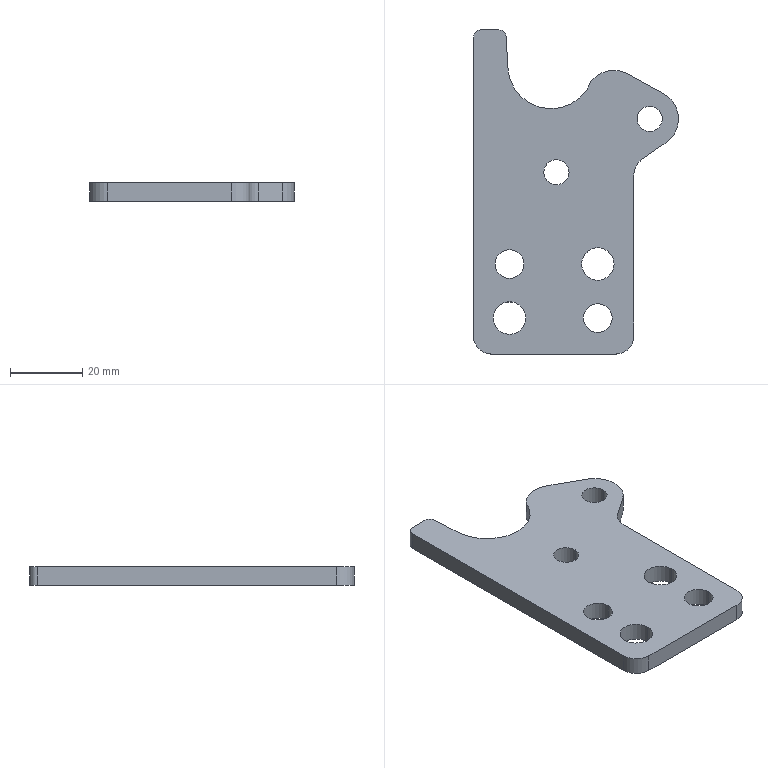Part | SolidWorks | features Fillet 2, Extrusion 1 | 1 solid | 29 faces | box 56.9 x 90 x 5 mm | volume 16455 mm3 | cylinder 20 | plane 9 | commonest cylinder face diameters 7 x4 8 x4 9 x4 4 x2 10 x2 16 x2
STEP:
#1=CARTESIAN_POINT('',(19.5,50.5,5.));
#2=VERTEX_POINT('',#1);
#3=CARTESIAN_POINT('',(26.5,50.5,5.));
#4=VERTEX_POINT('',#3);
#5=CARTESIAN_POINT('',(23.,50.5,5.));
#6=DIRECTION('',(0.,0.,1.));
#7=DIRECTION('',(1.,0.,0.));
#8=AXIS2_PLACEMENT_3D('',#5,#6,#7);
#9=CIRCLE('',#8,3.5);
#10=EDGE_CURVE('',#2,#4,#9,.T.);
#11=ORIENTED_EDGE('',*,*,#10,.T.);
#12=CARTESIAN_POINT('',(26.5,50.5,0.));
#13=VERTEX_POINT('',#12);
#14=CARTESIAN_POINT('',(26.5,50.5,5.));
#15=DIRECTION('',(0.,0.,-1.));
#16=VECTOR('',#15,1000.);
#17=LINE('',#14,#16);
#18=EDGE_CURVE('',#4,#13,#17,.T.);
#19=ORIENTED_EDGE('',*,*,#18,.T.);
#20=CARTESIAN_POINT('',(19.5,50.5,0.));
#21=VERTEX_POINT('',#20);
#22=CARTESIAN_POINT('',(23.,50.5,0.));
#23=DIRECTION('',(0.,0.,1.));
#24=DIRECTION('',(1.,0.,0.));
#25=AXIS2_PLACEMENT_3D('',#22,#23,#24);
#26=CIRCLE('',#25,3.5);
#27=EDGE_CURVE('',#21,#13,#26,.T.);
#28=ORIENTED_EDGE('',*,*,#27,.F.);
#29=CARTESIAN_POINT('',(19.5,50.5,5.));
#30=DIRECTION('',(0.,0.,-1.));
#31=VECTOR('',#30,1000.);
#32=LINE('',#29,#31);
#33=EDGE_CURVE('',#2,#21,#32,.T.);
#34=ORIENTED_EDGE('',*,*,#33,.F.);
#35=EDGE_LOOP('',(#11,#19,#28,#34));
#36=FACE_OUTER_BOUND('',#35,.T.);
#37=CARTESIAN_POINT('',(23.,50.5,5.));
#38=DIRECTION('',(0.,0.,-1.));
#39=DIRECTION('',(-1.,0.,0.));
#40=AXIS2_PLACEMENT_3D('',#37,#38,#39);
#41=CYLINDRICAL_SURFACE('',#40,3.5);
#42=ADVANCED_FACE('',(#36),#41,.F.);
#43=CARTESIAN_POINT('',(30.,25.,5.));
#44=VERTEX_POINT('',#43);
#45=CARTESIAN_POINT('',(39.,25.,5.));
#46=VERTEX_POINT('',#45);
#47=CARTESIAN_POINT('',(34.5,25.,5.));
#48=DIRECTION('',(0.,0.,1.));
#49=DIRECTION('',(1.,0.,0.));
#50=AXIS2_PLACEMENT_3D('',#47,#48,#49);
#51=CIRCLE('',#50,4.5);
#52=EDGE_CURVE('',#44,#46,#51,.T.);
#53=ORIENTED_EDGE('',*,*,#52,.T.);
#54=CARTESIAN_POINT('',(39.,25.,0.));
#55=VERTEX_POINT('',#54);
#56=CARTESIAN_POINT('',(39.,25.,5.));
#57=DIRECTION('',(0.,0.,-1.));
#58=VECTOR('',#57,1000.);
#59=LINE('',#56,#58);
#60=EDGE_CURVE('',#46,#55,#59,.T.);
#61=ORIENTED_EDGE('',*,*,#60,.T.);
#62=CARTESIAN_POINT('',(30.,25.,0.));
#63=VERTEX_POINT('',#62);
#64=CARTESIAN_POINT('',(34.5,25.,0.));
#65=DIRECTION('',(0.,0.,1.));
#66=DIRECTION('',(1.,0.,0.));
#67=AXIS2_PLACEMENT_3D('',#64,#65,#66);
#68=CIRCLE('',#67,4.5);
#69=EDGE_CURVE('',#63,#55,#68,.T.);
#70=ORIENTED_EDGE('',*,*,#69,.F.);
#71=CARTESIAN_POINT('',(30.,25.,5.));
#72=DIRECTION('',(0.,0.,-1.));
#73=VECTOR('',#72,1000.);
#74=LINE('',#71,#73);
#75=EDGE_CURVE('',#44,#63,#74,.T.);
#76=ORIENTED_EDGE('',*,*,#75,.F.);
#77=EDGE_LOOP('',(#53,#61,#70,#76));
#78=FACE_OUTER_BOUND('',#77,.T.);
#79=CARTESIAN_POINT('',(34.5,25.,5.));
#80=DIRECTION('',(0.,0.,-1.));
#81=DIRECTION('',(-1.,0.,0.));
#82=AXIS2_PLACEMENT_3D('',#79,#80,#81);
#83=CYLINDRICAL_SURFACE('',#82,4.5);
#84=ADVANCED_FACE('',(#78),#83,.F.);
#85=CARTESIAN_POINT('',(30.5,10.,5.));
#86=VERTEX_POINT('',#85);
#87=CARTESIAN_POINT('',(38.5,10.,5.));
#88=VERTEX_POINT('',#87);
#89=CARTESIAN_POINT('',(34.5,10.,5.));
#90=DIRECTION('',(0.,0.,1.));
#91=DIRECTION('',(1.,0.,0.));
#92=AXIS2_PLACEMENT_3D('',#89,#90,#91);
#93=CIRCLE('',#92,4.);
#94=EDGE_CURVE('',#86,#88,#93,.T.);
#95=ORIENTED_EDGE('',*,*,#94,.T.);
#96=CARTESIAN_POINT('',(38.5,10.,0.));
#97=VERTEX_POINT('',#96);
#98=CARTESIAN_POINT('',(38.5,10.,5.));
#99=DIRECTION('',(0.,0.,-1.));
#100=VECTOR('',#99,1000.);
#101=LINE('',#98,#100);
#102=EDGE_CURVE('',#88,#97,#101,.T.);
#103=ORIENTED_EDGE('',*,*,#102,.T.);
#104=CARTESIAN_POINT('',(30.5,10.,0.));
#105=VERTEX_POINT('',#104);
#106=CARTESIAN_POINT('',(34.5,10.,0.));
#107=DIRECTION('',(0.,0.,1.));
#108=DIRECTION('',(1.,0.,0.));
#109=AXIS2_PLACEMENT_3D('',#106,#107,#108);
#110=CIRCLE('',#109,4.);
#111=EDGE_CURVE('',#105,#97,#110,.T.);
#112=ORIENTED_EDGE('',*,*,#111,.F.);
#113=CARTESIAN_POINT('',(30.5,10.,5.));
#114=DIRECTION('',(0.,0.,-1.));
#115=VECTOR('',#114,1000.);
#116=LINE('',#113,#115);
#117=EDGE_CURVE('',#86,#105,#116,.T.);
#118=ORIENTED_EDGE('',*,*,#117,.F.);
#119=EDGE_LOOP('',(#95,#103,#112,#118));
#120=FACE_OUTER_BOUND('',#119,.T.);
#121=CARTESIAN_POINT('',(34.5,10.,5.));
#122=DIRECTION('',(0.,0.,-1.));
#123=DIRECTION('',(-1.,0.,0.));
#124=AXIS2_PLACEMENT_3D('',#121,#122,#123);
#125=CYLINDRICAL_SURFACE('',#124,4.);
#126=ADVANCED_FACE('',(#120),#125,.F.);
#127=CARTESIAN_POINT('',(6.,25.,5.));
#128=VERTEX_POINT('',#127);
#129=CARTESIAN_POINT('',(14.,25.,5.));
#130=VERTEX_POINT('',#129);
#131=CARTESIAN_POINT('',(10.,25.,5.));
#132=DIRECTION('',(0.,0.,1.));
#133=DIRECTION('',(1.,0.,0.));
#134=AXIS2_PLACEMENT_3D('',#131,#132,#133);
#135=CIRCLE('',#134,4.);
#136=EDGE_CURVE('',#128,#130,#135,.T.);
#137=ORIENTED_EDGE('',*,*,#136,.T.);
#138=CARTESIAN_POINT('',(14.,25.,0.));
#139=VERTEX_POINT('',#138);
#140=CARTESIAN_POINT('',(14.,25.,5.));
#141=DIRECTION('',(0.,0.,-1.));
#142=VECTOR('',#141,1000.);
#143=LINE('',#140,#142);
#144=EDGE_CURVE('',#130,#139,#143,.T.);
#145=ORIENTED_EDGE('',*,*,#144,.T.);
#146=CARTESIAN_POINT('',(6.,25.,0.));
#147=VERTEX_POINT('',#146);
#148=CARTESIAN_POINT('',(10.,25.,0.));
#149=DIRECTION('',(0.,0.,1.));
#150=DIRECTION('',(1.,0.,0.));
#151=AXIS2_PLACEMENT_3D('',#148,#149,#150);
#152=CIRCLE('',#151,4.);
#153=EDGE_CURVE('',#147,#139,#152,.T.);
#154=ORIENTED_EDGE('',*,*,#153,.F.);
#155=CARTESIAN_POINT('',(6.,25.,5.));
#156=DIRECTION('',(0.,0.,-1.));
#157=VECTOR('',#156,1000.);
#158=LINE('',#155,#157);
#159=EDGE_CURVE('',#128,#147,#158,.T.);
#160=ORIENTED_EDGE('',*,*,#159,.F.);
#161=EDGE_LOOP('',(#137,#145,#154,#160));
#162=FACE_OUTER_BOUND('',#161,.T.);
#163=CARTESIAN_POINT('',(10.,25.,5.));
#164=DIRECTION('',(0.,0.,-1.));
#165=DIRECTION('',(-1.,0.,0.));
#166=AXIS2_PLACEMENT_3D('',#163,#164,#165);
#167=CYLINDRICAL_SURFACE('',#166,4.);
#168=ADVANCED_FACE('',(#162),#167,.F.);
#169=CARTESIAN_POINT('',(5.5,10.,5.));
#170=VERTEX_POINT('',#169);
#171=CARTESIAN_POINT('',(14.5,10.,5.));
#172=VERTEX_POINT('',#171);
#173=CARTESIAN_POINT('',(10.,10.,5.));
#174=DIRECTION('',(0.,0.,1.));
#175=DIRECTION('',(1.,0.,0.));
#176=AXIS2_PLACEMENT_3D('',#173,#174,#175);
#177=CIRCLE('',#176,4.5);
#178=EDGE_CURVE('',#170,#172,#177,.T.);
#179=ORIENTED_EDGE('',*,*,#178,.T.);
#180=CARTESIAN_POINT('',(14.5,10.,0.));
#181=VERTEX_POINT('',#180);
#182=CARTESIAN_POINT('',(14.5,10.,5.));
#183=DIRECTION('',(0.,0.,-1.));
#184=VECTOR('',#183,1000.);
#185=LINE('',#182,#184);
#186=EDGE_CURVE('',#172,#181,#185,.T.);
#187=ORIENTED_EDGE('',*,*,#186,.T.);
#188=CARTESIAN_POINT('',(5.5,10.,0.));
#189=VERTEX_POINT('',#188);
#190=CARTESIAN_POINT('',(10.,10.,0.));
#191=DIRECTION('',(0.,0.,1.));
#192=DIRECTION('',(1.,0.,0.));
#193=AXIS2_PLACEMENT_3D('',#190,#191,#192);
#194=CIRCLE('',#193,4.5);
#195=EDGE_CURVE('',#189,#181,#194,.T.);
#196=ORIENTED_EDGE('',*,*,#195,.F.);
#197=CARTESIAN_POINT('',(5.5,10.,5.));
#198=DIRECTION('',(0.,0.,-1.));
#199=VECTOR('',#198,1000.);
#200=LINE('',#197,#199);
#201=EDGE_CURVE('',#170,#189,#200,.T.);
#202=ORIENTED_EDGE('',*,*,#201,.F.);
#203=EDGE_LOOP('',(#179,#187,#196,#202));
#204=FACE_OUTER_BOUND('',#203,.T.);
#205=CARTESIAN_POINT('',(10.,10.,5.));
#206=DIRECTION('',(0.,0.,-1.));
#207=DIRECTION('',(-1.,0.,0.));
#208=AXIS2_PLACEMENT_3D('',#205,#206,#207);
#209=CYLINDRICAL_SURFACE('',#208,4.5);
#210=ADVANCED_FACE('',(#204),#209,.F.);
#211=CARTESIAN_POINT('',(45.4,65.3,5.));
#212=VERTEX_POINT('',#211);
#213=CARTESIAN_POINT('',(52.4,65.3,5.));
#214=VERTEX_POINT('',#213);
#215=CARTESIAN_POINT('',(48.9,65.3,5.));
#216=DIRECTION('',(0.,0.,1.));
#217=DIRECTION('',(1.,0.,0.));
#218=AXIS2_PLACEMENT_3D('',#215,#216,#217);
#219=CIRCLE('',#218,3.5);
#220=EDGE_CURVE('',#212,#214,#219,.T.);
#221=ORIENTED_EDGE('',*,*,#220,.T.);
#222=CARTESIAN_POINT('',(52.4,65.3,0.));
#223=VERTEX_POINT('',#222);
#224=CARTESIAN_POINT('',(52.4,65.3,5.));
#225=DIRECTION('',(0.,0.,-1.));
#226=VECTOR('',#225,1000.);
#227=LINE('',#224,#226);
#228=EDGE_CURVE('',#214,#223,#227,.T.);
#229=ORIENTED_EDGE('',*,*,#228,.T.);
#230=CARTESIAN_POINT('',(45.4,65.3,0.));
#231=VERTEX_POINT('',#230);
#232=CARTESIAN_POINT('',(48.9,65.3,0.));
#233=DIRECTION('',(0.,0.,1.));
#234=DIRECTION('',(1.,0.,0.));
#235=AXIS2_PLACEMENT_3D('',#232,#233,#234);
#236=CIRCLE('',#235,3.5);
#237=EDGE_CURVE('',#231,#223,#236,.T.);
#238=ORIENTED_EDGE('',*,*,#237,.F.);
#239=CARTESIAN_POINT('',(45.4,65.3,5.));
#240=DIRECTION('',(0.,0.,-1.));
#241=VECTOR('',#240,1000.);
#242=LINE('',#239,#241);
#243=EDGE_CURVE('',#212,#231,#242,.T.);
#244=ORIENTED_EDGE('',*,*,#243,.F.);
#245=EDGE_LOOP('',(#221,#229,#238,#244));
#246=FACE_OUTER_BOUND('',#245,.T.);
#247=CARTESIAN_POINT('',(48.9,65.3,5.));
#248=DIRECTION('',(0.,0.,-1.));
#249=DIRECTION('',(-1.,0.,0.));
#250=AXIS2_PLACEMENT_3D('',#247,#248,#249);
#251=CYLINDRICAL_SURFACE('',#250,3.5);
#252=ADVANCED_FACE('',(#246),#251,.F.);
#253=ORIENTED_EDGE('',*,*,#52,.F.);
#254=CARTESIAN_POINT('',(34.5,25.,5.));
#255=DIRECTION('',(0.,0.,1.));
#256=DIRECTION('',(1.,0.,0.));
#257=AXIS2_PLACEMENT_3D('',#254,#255,#256);
#258=CIRCLE('',#257,4.5);
#259=EDGE_CURVE('',#46,#44,#258,.T.);
#260=ORIENTED_EDGE('',*,*,#259,.F.);
#261=EDGE_LOOP('',(#253,#260));
#262=FACE_BOUND('',#261,.T.);
#263=ORIENTED_EDGE('',*,*,#136,.F.);
#264=CARTESIAN_POINT('',(10.,25.,5.));
#265=DIRECTION('',(0.,0.,1.));
#266=DIRECTION('',(1.,0.,0.));
#267=AXIS2_PLACEMENT_3D('',#264,#265,#266);
#268=CIRCLE('',#267,4.);
#269=EDGE_CURVE('',#130,#128,#268,.T.);
#270=ORIENTED_EDGE('',*,*,#269,.F.);
#271=EDGE_LOOP('',(#263,#270));
#272=FACE_BOUND('',#271,.T.);
#273=ORIENTED_EDGE('',*,*,#220,.F.);
#274=CARTESIAN_POINT('',(48.9,65.3,5.));
#275=DIRECTION('',(0.,0.,1.));
#276=DIRECTION('',(1.,0.,0.));
#277=AXIS2_PLACEMENT_3D('',#274,#275,#276);
#278=CIRCLE('',#277,3.5);
#279=EDGE_CURVE('',#214,#212,#278,.T.);
#280=ORIENTED_EDGE('',*,*,#279,.F.);
#281=EDGE_LOOP('',(#273,#280));
#282=FACE_BOUND('',#281,.T.);
#283=CARTESIAN_POINT('',(5.,0.,5.));
#284=VERTEX_POINT('',#283);
#285=CARTESIAN_POINT('',(39.5,0.,5.));
#286=VERTEX_POINT('',#285);
#287=CARTESIAN_POINT('',(0.,0.,5.));
#288=DIRECTION('',(1.,0.,0.));
#289=VECTOR('',#288,1000.);
#290=LINE('',#287,#289);
#291=EDGE_CURVE('',#284,#286,#290,.T.);
#292=ORIENTED_EDGE('',*,*,#291,.T.);
#293=CARTESIAN_POINT('',(44.5,5.,5.));
#294=VERTEX_POINT('',#293);
#295=CARTESIAN_POINT('',(39.5,5.,5.));
#296=DIRECTION('',(0.,0.,1.));
#297=DIRECTION('',(1.,0.,0.));
#298=AXIS2_PLACEMENT_3D('',#295,#296,#297);
#299=CIRCLE('',#298,5.);
#300=EDGE_CURVE('',#286,#294,#299,.T.);
#301=ORIENTED_EDGE('',*,*,#300,.T.);
#302=CARTESIAN_POINT('',(44.5,49.666,5.));
#303=VERTEX_POINT('',#302);
#304=CARTESIAN_POINT('',(44.5,0.,5.));
#305=DIRECTION('',(0.,1.,0.));
#306=VECTOR('',#305,1000.);
#307=LINE('',#304,#306);
#308=EDGE_CURVE('',#294,#303,#307,.T.);
#309=ORIENTED_EDGE('',*,*,#308,.T.);
#310=CARTESIAN_POINT('',(46.881,54.196,5.));
#311=VERTEX_POINT('',#310);
#312=CARTESIAN_POINT('',(50.,49.666,5.));
#313=DIRECTION('',(0.,0.,-1.));
#314=DIRECTION('',(1.,0.,0.));
#315=AXIS2_PLACEMENT_3D('',#312,#313,#314);
#316=CIRCLE('',#315,5.5);
#317=EDGE_CURVE('',#303,#311,#316,.T.);
#318=ORIENTED_EDGE('',*,*,#317,.T.);
#319=CARTESIAN_POINT('',(53.437,58.711,5.));
#320=VERTEX_POINT('',#319);
#321=CARTESIAN_POINT('',(53.437,58.711,5.));
#322=DIRECTION('',(0.8236,0.5672,0.));
#323=VECTOR('',#322,1000.);
#324=LINE('',#321,#323);
#325=EDGE_CURVE('',#311,#320,#324,.T.);
#326=ORIENTED_EDGE('',*,*,#325,.T.);
#327=CARTESIAN_POINT('',(52.755,72.31,5.));
#328=VERTEX_POINT('',#327);
#329=CARTESIAN_POINT('',(48.9,65.3,5.));
#330=DIRECTION('',(0.,0.,1.));
#331=DIRECTION('',(1.,0.,0.));
#332=AXIS2_PLACEMENT_3D('',#329,#330,#331);
#333=CIRCLE('',#332,8.);
#334=EDGE_CURVE('',#320,#328,#333,.T.);
#335=ORIENTED_EDGE('',*,*,#334,.T.);
#336=CARTESIAN_POINT('',(42.755,77.81,5.));
#337=VERTEX_POINT('',#336);
#338=CARTESIAN_POINT('',(42.755,77.81,5.));
#339=DIRECTION('',(-0.8762,0.4819,0.));
#340=VECTOR('',#339,1000.);
#341=LINE('',#338,#340);
#342=EDGE_CURVE('',#328,#337,#341,.T.);
#343=ORIENTED_EDGE('',*,*,#342,.T.);
#344=CARTESIAN_POINT('',(32.745,75.91,5.));
#345=VERTEX_POINT('',#344);
#346=CARTESIAN_POINT('',(38.9,70.8,5.));
#347=DIRECTION('',(0.,0.,1.));
#348=DIRECTION('',(1.,0.,0.));
#349=AXIS2_PLACEMENT_3D('',#346,#347,#348);
#350=CIRCLE('',#349,8.);
#351=EDGE_CURVE('',#337,#345,#350,.T.);
#352=ORIENTED_EDGE('',*,*,#351,.T.);
#353=CARTESIAN_POINT('',(9.516,79.472,5.));
#354=VERTEX_POINT('',#353);
#355=CARTESIAN_POINT('',(21.5,80.1,5.));
#356=DIRECTION('',(0.,0.,-1.));
#357=DIRECTION('',(1.,0.,0.));
#358=AXIS2_PLACEMENT_3D('',#355,#356,#357);
#359=CIRCLE('',#358,12.);
#360=EDGE_CURVE('',#345,#354,#359,.T.);
#361=ORIENTED_EDGE('',*,*,#360,.T.);
#362=CARTESIAN_POINT('',(9.064,88.105,5.));
#363=VERTEX_POINT('',#362);
#364=CARTESIAN_POINT('',(8.965,90.,5.));
#365=DIRECTION('',(-0.05234,0.9986,0.));
#366=VECTOR('',#365,1000.);
#367=LINE('',#364,#366);
#368=EDGE_CURVE('',#354,#363,#367,.T.);
#369=ORIENTED_EDGE('',*,*,#368,.T.);
#370=CARTESIAN_POINT('',(7.067,90.,5.));
#371=VERTEX_POINT('',#370);
#372=CARTESIAN_POINT('',(7.067,88.,5.));
#373=DIRECTION('',(0.,0.,1.));
#374=DIRECTION('',(1.,0.,0.));
#375=AXIS2_PLACEMENT_3D('',#372,#373,#374);
#376=CIRCLE('',#375,2.);
#377=EDGE_CURVE('',#363,#371,#376,.T.);
#378=ORIENTED_EDGE('',*,*,#377,.T.);
#379=CARTESIAN_POINT('',(2.,90.,5.));
#380=VERTEX_POINT('',#379);
#381=CARTESIAN_POINT('',(0.,90.,5.));
#382=DIRECTION('',(-1.,0.,0.));
#383=VECTOR('',#382,1000.);
#384=LINE('',#381,#383);
#385=EDGE_CURVE('',#371,#380,#384,.T.);
#386=ORIENTED_EDGE('',*,*,#385,.T.);
#387=CARTESIAN_POINT('',(0.,88.,5.));
#388=VERTEX_POINT('',#387);
#389=CARTESIAN_POINT('',(2.,88.,5.));
#390=DIRECTION('',(0.,0.,1.));
#391=DIRECTION('',(1.,0.,0.));
#392=AXIS2_PLACEMENT_3D('',#389,#390,#391);
#393=CIRCLE('',#392,2.);
#394=EDGE_CURVE('',#380,#388,#393,.T.);
#395=ORIENTED_EDGE('',*,*,#394,.T.);
#396=CARTESIAN_POINT('',(0.,5.,5.));
#397=VERTEX_POINT('',#396);
#398=CARTESIAN_POINT('',(0.,0.,5.));
#399=DIRECTION('',(0.,-1.,0.));
#400=VECTOR('',#399,1000.);
#401=LINE('',#398,#400);
#402=EDGE_CURVE('',#388,#397,#401,.T.);
#403=ORIENTED_EDGE('',*,*,#402,.T.);
#404=CARTESIAN_POINT('',(5.,5.,5.));
#405=DIRECTION('',(0.,0.,1.));
#406=DIRECTION('',(1.,0.,0.));
#407=AXIS2_PLACEMENT_3D('',#404,#405,#406);
#408=CIRCLE('',#407,5.);
#409=EDGE_CURVE('',#397,#284,#408,.T.);
#410=ORIENTED_EDGE('',*,*,#409,.T.);
#411=EDGE_LOOP('',(#292,#301,#309,#318,#326,#335,#343,#352,#361,#369,#378,#386,#395,#403,#410));
#412=FACE_OUTER_BOUND('',#411,.T.);
#413=ORIENTED_EDGE('',*,*,#178,.F.);
#414=CARTESIAN_POINT('',(10.,10.,5.));
#415=DIRECTION('',(0.,0.,1.));
#416=DIRECTION('',(1.,0.,0.));
#417=AXIS2_PLACEMENT_3D('',#414,#415,#416);
#418=CIRCLE('',#417,4.5);
#419=EDGE_CURVE('',#172,#170,#418,.T.);
#420=ORIENTED_EDGE('',*,*,#419,.F.);
#421=EDGE_LOOP('',(#413,#420));
#422=FACE_BOUND('',#421,.T.);
#423=ORIENTED_EDGE('',*,*,#94,.F.);
#424=CARTESIAN_POINT('',(34.5,10.,5.));
#425=DIRECTION('',(0.,0.,1.));
#426=DIRECTION('',(1.,0.,0.));
#427=AXIS2_PLACEMENT_3D('',#424,#425,#426);
#428=CIRCLE('',#427,4.);
#429=EDGE_CURVE('',#88,#86,#428,.T.);
#430=ORIENTED_EDGE('',*,*,#429,.F.);
#431=EDGE_LOOP('',(#423,#430));
#432=FACE_BOUND('',#431,.T.);
#433=ORIENTED_EDGE('',*,*,#10,.F.);
#434=CARTESIAN_POINT('',(23.,50.5,5.));
#435=DIRECTION('',(0.,0.,1.));
#436=DIRECTION('',(1.,0.,0.));
#437=AXIS2_PLACEMENT_3D('',#434,#435,#436);
#438=CIRCLE('',#437,3.5);
#439=EDGE_CURVE('',#4,#2,#438,.T.);
#440=ORIENTED_EDGE('',*,*,#439,.F.);
#441=EDGE_LOOP('',(#433,#440));
#442=FACE_BOUND('',#441,.T.);
#443=CARTESIAN_POINT('',(21.5,80.1,5.));
#444=DIRECTION('',(0.,0.,1.));
#445=DIRECTION('',(1.,0.,0.));
#446=AXIS2_PLACEMENT_3D('',#443,#444,#445);
#447=PLANE('',#446);
#448=ADVANCED_FACE('',(#262,#272,#282,#412,#422,#432,#442),#447,.T.);
#449=CARTESIAN_POINT('',(44.5,5.,0.));
#450=VERTEX_POINT('',#449);
#451=CARTESIAN_POINT('',(44.5,49.666,0.));
#452=VERTEX_POINT('',#451);
#453=CARTESIAN_POINT('',(44.5,0.,0.));
#454=DIRECTION('',(0.,1.,0.));
#455=VECTOR('',#454,1000.);
#456=LINE('',#453,#455);
#457=EDGE_CURVE('',#450,#452,#456,.T.);
#458=ORIENTED_EDGE('',*,*,#457,.F.);
#459=CARTESIAN_POINT('',(39.5,0.,0.));
#460=VERTEX_POINT('',#459);
#461=CARTESIAN_POINT('',(39.5,5.,0.));
#462=DIRECTION('',(0.,0.,-1.));
#463=DIRECTION('',(1.,0.,0.));
#464=AXIS2_PLACEMENT_3D('',#461,#462,#463);
#465=CIRCLE('',#464,5.);
#466=EDGE_CURVE('',#450,#460,#465,.T.);
#467=ORIENTED_EDGE('',*,*,#466,.T.);
#468=CARTESIAN_POINT('',(5.,0.,0.));
#469=VERTEX_POINT('',#468);
#470=CARTESIAN_POINT('',(0.,0.,0.));
#471=DIRECTION('',(1.,0.,0.));
#472=VECTOR('',#471,1000.);
#473=LINE('',#470,#472);
#474=EDGE_CURVE('',#469,#460,#473,.T.);
#475=ORIENTED_EDGE('',*,*,#474,.F.);
#476=CARTESIAN_POINT('',(0.,5.,0.));
#477=VERTEX_POINT('',#476);
#478=CARTESIAN_POINT('',(5.,5.,0.));
#479=DIRECTION('',(0.,0.,-1.));
#480=DIRECTION('',(1.,0.,0.));
#481=AXIS2_PLACEMENT_3D('',#478,#479,#480);
#482=CIRCLE('',#481,5.);
#483=EDGE_CURVE('',#469,#477,#482,.T.);
#484=ORIENTED_EDGE('',*,*,#483,.T.);
#485=CARTESIAN_POINT('',(0.,88.,0.));
#486=VERTEX_POINT('',#485);
#487=CARTESIAN_POINT('',(0.,0.,0.));
#488=DIRECTION('',(0.,-1.,0.));
#489=VECTOR('',#488,1000.);
#490=LINE('',#487,#489);
#491=EDGE_CURVE('',#486,#477,#490,.T.);
#492=ORIENTED_EDGE('',*,*,#491,.F.);
#493=CARTESIAN_POINT('',(2.,90.,0.));
#494=VERTEX_POINT('',#493);
#495=CARTESIAN_POINT('',(2.,88.,0.));
#496=DIRECTION('',(0.,0.,-1.));
#497=DIRECTION('',(1.,0.,0.));
#498=AXIS2_PLACEMENT_3D('',#495,#496,#497);
#499=CIRCLE('',#498,2.);
#500=EDGE_CURVE('',#486,#494,#499,.T.);
#501=ORIENTED_EDGE('',*,*,#500,.T.);
#502=CARTESIAN_POINT('',(7.067,90.,0.));
#503=VERTEX_POINT('',#502);
#504=CARTESIAN_POINT('',(0.,90.,0.));
#505=DIRECTION('',(-1.,0.,0.));
#506=VECTOR('',#505,1000.);
#507=LINE('',#504,#506);
#508=EDGE_CURVE('',#503,#494,#507,.T.);
#509=ORIENTED_EDGE('',*,*,#508,.F.);
#510=CARTESIAN_POINT('',(9.064,88.105,0.));
#511=VERTEX_POINT('',#510);
#512=CARTESIAN_POINT('',(7.067,88.,0.));
#513=DIRECTION('',(0.,0.,-1.));
#514=DIRECTION('',(1.,0.,0.));
#515=AXIS2_PLACEMENT_3D('',#512,#513,#514);
#516=CIRCLE('',#515,2.);
#517=EDGE_CURVE('',#503,#511,#516,.T.);
#518=ORIENTED_EDGE('',*,*,#517,.T.);
#519=CARTESIAN_POINT('',(9.516,79.472,0.));
#520=VERTEX_POINT('',#519);
#521=CARTESIAN_POINT('',(8.965,90.,0.));
#522=DIRECTION('',(-0.05234,0.9986,0.));
#523=VECTOR('',#522,1000.);
#524=LINE('',#521,#523);
#525=EDGE_CURVE('',#520,#511,#524,.T.);
#526=ORIENTED_EDGE('',*,*,#525,.F.);
#527=CARTESIAN_POINT('',(32.745,75.91,0.));
#528=VERTEX_POINT('',#527);
#529=CARTESIAN_POINT('',(21.5,80.1,0.));
#530=DIRECTION('',(0.,0.,-1.));
#531=DIRECTION('',(1.,0.,0.));
#532=AXIS2_PLACEMENT_3D('',#529,#530,#531);
#533=CIRCLE('',#532,12.);
#534=EDGE_CURVE('',#528,#520,#533,.T.);
#535=ORIENTED_EDGE('',*,*,#534,.F.);
#536=CARTESIAN_POINT('',(42.755,77.81,0.));
#537=VERTEX_POINT('',#536);
#538=CARTESIAN_POINT('',(38.9,70.8,0.));
#539=DIRECTION('',(0.,0.,1.));
#540=DIRECTION('',(1.,0.,0.));
#541=AXIS2_PLACEMENT_3D('',#538,#539,#540);
#542=CIRCLE('',#541,8.);
#543=EDGE_CURVE('',#537,#528,#542,.T.);
#544=ORIENTED_EDGE('',*,*,#543,.F.);
#545=CARTESIAN_POINT('',(52.755,72.31,0.));
#546=VERTEX_POINT('',#545);
#547=CARTESIAN_POINT('',(42.755,77.81,0.));
#548=DIRECTION('',(-0.8762,0.4819,0.));
#549=VECTOR('',#548,1000.);
#550=LINE('',#547,#549);
#551=EDGE_CURVE('',#546,#537,#550,.T.);
#552=ORIENTED_EDGE('',*,*,#551,.F.);
#553=CARTESIAN_POINT('',(53.437,58.711,0.));
#554=VERTEX_POINT('',#553);
#555=CARTESIAN_POINT('',(48.9,65.3,0.));
#556=DIRECTION('',(0.,0.,1.));
#557=DIRECTION('',(1.,0.,0.));
#558=AXIS2_PLACEMENT_3D('',#555,#556,#557);
#559=CIRCLE('',#558,8.);
#560=EDGE_CURVE('',#554,#546,#559,.T.);
#561=ORIENTED_EDGE('',*,*,#560,.F.);
#562=CARTESIAN_POINT('',(46.881,54.196,0.));
#563=VERTEX_POINT('',#562);
#564=CARTESIAN_POINT('',(53.437,58.711,0.));
#565=DIRECTION('',(0.8236,0.5672,0.));
#566=VECTOR('',#565,1000.);
#567=LINE('',#564,#566);
#568=EDGE_CURVE('',#563,#554,#567,.T.);
#569=ORIENTED_EDGE('',*,*,#568,.F.);
#570=CARTESIAN_POINT('',(50.,49.666,0.));
#571=DIRECTION('',(0.,0.,-1.));
#572=DIRECTION('',(1.,0.,0.));
#573=AXIS2_PLACEMENT_3D('',#570,#571,#572);
#574=CIRCLE('',#573,5.5);
#575=EDGE_CURVE('',#452,#563,#574,.T.);
#576=ORIENTED_EDGE('',*,*,#575,.F.);
#577=EDGE_LOOP('',(#458,#467,#475,#484,#492,#501,#509,#518,#526,#535,#544,#552,#561,#569,#576));
#578=FACE_OUTER_BOUND('',#577,.T.);
#579=ORIENTED_EDGE('',*,*,#237,.T.);
#580=CARTESIAN_POINT('',(48.9,65.3,0.));
#581=DIRECTION('',(0.,0.,1.));
#582=DIRECTION('',(1.,0.,0.));
#583=AXIS2_PLACEMENT_3D('',#580,#581,#582);
#584=CIRCLE('',#583,3.5);
#585=EDGE_CURVE('',#223,#231,#584,.T.);
#586=ORIENTED_EDGE('',*,*,#585,.T.);
#587=EDGE_LOOP('',(#579,#586));
#588=FACE_BOUND('',#587,.T.);
#589=ORIENTED_EDGE('',*,*,#195,.T.);
#590=CARTESIAN_POINT('',(10.,10.,0.));
#591=DIRECTION('',(0.,0.,1.));
#592=DIRECTION('',(1.,0.,0.));
#593=AXIS2_PLACEMENT_3D('',#590,#591,#592);
#594=CIRCLE('',#593,4.5);
#595=EDGE_CURVE('',#181,#189,#594,.T.);
#596=ORIENTED_EDGE('',*,*,#595,.T.);
#597=EDGE_LOOP('',(#589,#596));
#598=FACE_BOUND('',#597,.T.);
#599=ORIENTED_EDGE('',*,*,#153,.T.);
#600=CARTESIAN_POINT('',(10.,25.,0.));
#601=DIRECTION('',(0.,0.,1.));
#602=DIRECTION('',(1.,0.,0.));
#603=AXIS2_PLACEMENT_3D('',#600,#601,#602);
#604=CIRCLE('',#603,4.);
#605=EDGE_CURVE('',#139,#147,#604,.T.);
#606=ORIENTED_EDGE('',*,*,#605,.T.);
#607=EDGE_LOOP('',(#599,#606));
#608=FACE_BOUND('',#607,.T.);
#609=ORIENTED_EDGE('',*,*,#111,.T.);
#610=CARTESIAN_POINT('',(34.5,10.,0.));
#611=DIRECTION('',(0.,0.,1.));
#612=DIRECTION('',(1.,0.,0.));
#613=AXIS2_PLACEMENT_3D('',#610,#611,#612);
#614=CIRCLE('',#613,4.);
#615=EDGE_CURVE('',#97,#105,#614,.T.);
#616=ORIENTED_EDGE('',*,*,#615,.T.);
#617=EDGE_LOOP('',(#609,#616));
#618=FACE_BOUND('',#617,.T.);
#619=ORIENTED_EDGE('',*,*,#69,.T.);
#620=CARTESIAN_POINT('',(34.5,25.,0.));
#621=DIRECTION('',(0.,0.,1.));
#622=DIRECTION('',(1.,0.,0.));
#623=AXIS2_PLACEMENT_3D('',#620,#621,#622);
#624=CIRCLE('',#623,4.5);
#625=EDGE_CURVE('',#55,#63,#624,.T.);
#626=ORIENTED_EDGE('',*,*,#625,.T.);
#627=EDGE_LOOP('',(#619,#626));
#628=FACE_BOUND('',#627,.T.);
#629=ORIENTED_EDGE('',*,*,#27,.T.);
#630=CARTESIAN_POINT('',(23.,50.5,0.));
#631=DIRECTION('',(0.,0.,1.));
#632=DIRECTION('',(1.,0.,0.));
#633=AXIS2_PLACEMENT_3D('',#630,#631,#632);
#634=CIRCLE('',#633,3.5);
#635=EDGE_CURVE('',#13,#21,#634,.T.);
#636=ORIENTED_EDGE('',*,*,#635,.T.);
#637=EDGE_LOOP('',(#629,#636));
#638=FACE_BOUND('',#637,.T.);
#639=CARTESIAN_POINT('',(21.5,80.1,0.));
#640=DIRECTION('',(0.,0.,1.));
#641=DIRECTION('',(1.,0.,0.));
#642=AXIS2_PLACEMENT_3D('',#639,#640,#641);
#643=PLANE('',#642);
#644=ADVANCED_FACE('',(#578,#588,#598,#608,#618,#628,#638),#643,.F.);
#645=ORIENTED_EDGE('',*,*,#491,.T.);
#646=CARTESIAN_POINT('',(0.,5.,5.));
#647=DIRECTION('',(0.,0.,1.));
#648=VECTOR('',#647,1000.);
#649=LINE('',#646,#648);
#650=EDGE_CURVE('',#477,#397,#649,.T.);
#651=ORIENTED_EDGE('',*,*,#650,.T.);
#652=ORIENTED_EDGE('',*,*,#402,.F.);
#653=CARTESIAN_POINT('',(0.,88.,5.));
#654=DIRECTION('',(0.,0.,-1.));
#655=VECTOR('',#654,1000.);
#656=LINE('',#653,#655);
#657=EDGE_CURVE('',#388,#486,#656,.T.);
#658=ORIENTED_EDGE('',*,*,#657,.T.);
#659=EDGE_LOOP('',(#645,#651,#652,#658));
#660=FACE_OUTER_BOUND('',#659,.T.);
#661=CARTESIAN_POINT('',(0.,0.,5.));
#662=DIRECTION('',(1.,0.,0.));
#663=DIRECTION('',(0.,0.,-1.));
#664=AXIS2_PLACEMENT_3D('',#661,#662,#663);
#665=PLANE('',#664);
#666=ADVANCED_FACE('',(#660),#665,.F.);
#667=ORIENTED_EDGE('',*,*,#474,.T.);
#668=CARTESIAN_POINT('',(39.5,0.,5.));
#669=DIRECTION('',(0.,0.,1.));
#670=VECTOR('',#669,1000.);
#671=LINE('',#668,#670);
#672=EDGE_CURVE('',#460,#286,#671,.T.);
#673=ORIENTED_EDGE('',*,*,#672,.T.);
#674=ORIENTED_EDGE('',*,*,#291,.F.);
#675=CARTESIAN_POINT('',(5.,0.,5.));
#676=DIRECTION('',(0.,0.,-1.));
#677=VECTOR('',#676,1000.);
#678=LINE('',#675,#677);
#679=EDGE_CURVE('',#284,#469,#678,.T.);
#680=ORIENTED_EDGE('',*,*,#679,.T.);
#681=EDGE_LOOP('',(#667,#673,#674,#680));
#682=FACE_OUTER_BOUND('',#681,.T.);
#683=CARTESIAN_POINT('',(0.,0.,5.));
#684=DIRECTION('',(0.,1.,0.));
#685=DIRECTION('',(0.,0.,1.));
#686=AXIS2_PLACEMENT_3D('',#683,#684,#685);
#687=PLANE('',#686);
#688=ADVANCED_FACE('',(#682),#687,.F.);
#689=ORIENTED_EDGE('',*,*,#308,.F.);
#690=CARTESIAN_POINT('',(44.5,5.,5.));
#691=DIRECTION('',(0.,0.,-1.));
#692=VECTOR('',#691,1000.);
#693=LINE('',#690,#692);
#694=EDGE_CURVE('',#294,#450,#693,.T.);
#695=ORIENTED_EDGE('',*,*,#694,.T.);
#696=ORIENTED_EDGE('',*,*,#457,.T.);
#697=CARTESIAN_POINT('',(44.5,49.666,5.));
#698=DIRECTION('',(0.,0.,-1.));
#699=VECTOR('',#698,1000.);
#700=LINE('',#697,#699);
#701=EDGE_CURVE('',#303,#452,#700,.T.);
#702=ORIENTED_EDGE('',*,*,#701,.F.);
#703=EDGE_LOOP('',(#689,#695,#696,#702));
#704=FACE_OUTER_BOUND('',#703,.T.);
#705=CARTESIAN_POINT('',(44.5,0.,5.));
#706=DIRECTION('',(-1.,0.,0.));
#707=DIRECTION('',(0.,0.,1.));
#708=AXIS2_PLACEMENT_3D('',#705,#706,#707);
#709=PLANE('',#708);
#710=ADVANCED_FACE('',(#704),#709,.F.);
#711=ORIENTED_EDGE('',*,*,#575,.T.);
#712=CARTESIAN_POINT('',(46.881,54.196,5.));
#713=DIRECTION('',(0.,0.,-1.));
#714=VECTOR('',#713,1000.);
#715=LINE('',#712,#714);
#716=EDGE_CURVE('',#311,#563,#715,.T.);
#717=ORIENTED_EDGE('',*,*,#716,.F.);
#718=ORIENTED_EDGE('',*,*,#317,.F.);
#719=ORIENTED_EDGE('',*,*,#701,.T.);
#720=EDGE_LOOP('',(#711,#717,#718,#719));
#721=FACE_OUTER_BOUND('',#720,.T.);
#722=CARTESIAN_POINT('',(50.,49.666,5.));
#723=DIRECTION('',(0.,0.,-1.));
#724=DIRECTION('',(-1.,0.,0.));
#725=AXIS2_PLACEMENT_3D('',#722,#723,#724);
#726=CYLINDRICAL_SURFACE('',#725,5.5);
#727=ADVANCED_FACE('',(#721),#726,.F.);
#728=ORIENTED_EDGE('',*,*,#568,.T.);
#729=CARTESIAN_POINT('',(53.437,58.711,5.));
#730=DIRECTION('',(0.,0.,-1.));
#731=VECTOR('',#730,1000.);
#732=LINE('',#729,#731);
#733=EDGE_CURVE('',#320,#554,#732,.T.);
#734=ORIENTED_EDGE('',*,*,#733,.F.);
#735=ORIENTED_EDGE('',*,*,#325,.F.);
#736=ORIENTED_EDGE('',*,*,#716,.T.);
#737=EDGE_LOOP('',(#728,#734,#735,#736));
#738=FACE_OUTER_BOUND('',#737,.T.);
#739=CARTESIAN_POINT('',(53.437,58.711,5.));
#740=DIRECTION('',(-0.5672,0.8236,0.));
#741=DIRECTION('',(-0.8236,-0.5672,0.));
#742=AXIS2_PLACEMENT_3D('',#739,#740,#741);
#743=PLANE('',#742);
#744=ADVANCED_FACE('',(#738),#743,.F.);
#745=ORIENTED_EDGE('',*,*,#560,.T.);
#746=CARTESIAN_POINT('',(52.755,72.31,5.));
#747=DIRECTION('',(0.,0.,-1.));
#748=VECTOR('',#747,1000.);
#749=LINE('',#746,#748);
#750=EDGE_CURVE('',#328,#546,#749,.T.);
#751=ORIENTED_EDGE('',*,*,#750,.F.);
#752=ORIENTED_EDGE('',*,*,#334,.F.);
#753=ORIENTED_EDGE('',*,*,#733,.T.);
#754=EDGE_LOOP('',(#745,#751,#752,#753));
#755=FACE_OUTER_BOUND('',#754,.T.);
#756=CARTESIAN_POINT('',(48.9,65.3,5.));
#757=DIRECTION('',(0.,0.,-1.));
#758=DIRECTION('',(-1.,0.,0.));
#759=AXIS2_PLACEMENT_3D('',#756,#757,#758);
#760=CYLINDRICAL_SURFACE('',#759,8.);
#761=ADVANCED_FACE('',(#755),#760,.T.);
#762=ORIENTED_EDGE('',*,*,#551,.T.);
#763=CARTESIAN_POINT('',(42.755,77.81,5.));
#764=DIRECTION('',(0.,0.,-1.));
#765=VECTOR('',#764,1000.);
#766=LINE('',#763,#765);
#767=EDGE_CURVE('',#337,#537,#766,.T.);
#768=ORIENTED_EDGE('',*,*,#767,.F.);
#769=ORIENTED_EDGE('',*,*,#342,.F.);
#770=ORIENTED_EDGE('',*,*,#750,.T.);
#771=EDGE_LOOP('',(#762,#768,#769,#770));
#772=FACE_OUTER_BOUND('',#771,.T.);
#773=CARTESIAN_POINT('',(42.755,77.81,5.));
#774=DIRECTION('',(-0.4819,-0.8762,0.));
#775=DIRECTION('',(0.8762,-0.4819,0.));
#776=AXIS2_PLACEMENT_3D('',#773,#774,#775);
#777=PLANE('',#776);
#778=ADVANCED_FACE('',(#772),#777,.F.);
#779=ORIENTED_EDGE('',*,*,#543,.T.);
#780=CARTESIAN_POINT('',(32.745,75.91,5.));
#781=DIRECTION('',(0.,0.,-1.));
#782=VECTOR('',#781,1000.);
#783=LINE('',#780,#782);
#784=EDGE_CURVE('',#345,#528,#783,.T.);
#785=ORIENTED_EDGE('',*,*,#784,.F.);
#786=ORIENTED_EDGE('',*,*,#351,.F.);
#787=ORIENTED_EDGE('',*,*,#767,.T.);
#788=EDGE_LOOP('',(#779,#785,#786,#787));
#789=FACE_OUTER_BOUND('',#788,.T.);
#790=CARTESIAN_POINT('',(38.9,70.8,5.));
#791=DIRECTION('',(0.,0.,-1.));
#792=DIRECTION('',(-1.,0.,0.));
#793=AXIS2_PLACEMENT_3D('',#790,#791,#792);
#794=CYLINDRICAL_SURFACE('',#793,8.);
#795=ADVANCED_FACE('',(#789),#794,.T.);
#796=ORIENTED_EDGE('',*,*,#534,.T.);
#797=CARTESIAN_POINT('',(9.516,79.472,5.));
#798=DIRECTION('',(0.,0.,-1.));
#799=VECTOR('',#798,1000.);
#800=LINE('',#797,#799);
#801=EDGE_CURVE('',#354,#520,#800,.T.);
#802=ORIENTED_EDGE('',*,*,#801,.F.);
#803=ORIENTED_EDGE('',*,*,#360,.F.);
#804=ORIENTED_EDGE('',*,*,#784,.T.);
#805=EDGE_LOOP('',(#796,#802,#803,#804));
#806=FACE_OUTER_BOUND('',#805,.T.);
#807=CARTESIAN_POINT('',(21.5,80.1,5.));
#808=DIRECTION('',(0.,0.,-1.));
#809=DIRECTION('',(-1.,0.,0.));
#810=AXIS2_PLACEMENT_3D('',#807,#808,#809);
#811=CYLINDRICAL_SURFACE('',#810,12.);
#812=ADVANCED_FACE('',(#806),#811,.F.);
#813=ORIENTED_EDGE('',*,*,#525,.T.);
#814=CARTESIAN_POINT('',(9.064,88.105,5.));
#815=DIRECTION('',(0.,0.,1.));
#816=VECTOR('',#815,1000.);
#817=LINE('',#814,#816);
#818=EDGE_CURVE('',#511,#363,#817,.T.);
#819=ORIENTED_EDGE('',*,*,#818,.T.);
#820=ORIENTED_EDGE('',*,*,#368,.F.);
#821=ORIENTED_EDGE('',*,*,#801,.T.);
#822=EDGE_LOOP('',(#813,#819,#820,#821));
#823=FACE_OUTER_BOUND('',#822,.T.);
#824=CARTESIAN_POINT('',(8.965,90.,5.));
#825=DIRECTION('',(-0.9986,-0.05234,0.));
#826=DIRECTION('',(0.05234,-0.9986,0.));
#827=AXIS2_PLACEMENT_3D('',#824,#825,#826);
#828=PLANE('',#827);
#829=ADVANCED_FACE('',(#823),#828,.F.);
#830=ORIENTED_EDGE('',*,*,#385,.F.);
#831=CARTESIAN_POINT('',(7.067,90.,5.));
#832=DIRECTION('',(0.,0.,-1.));
#833=VECTOR('',#832,1000.);
#834=LINE('',#831,#833);
#835=EDGE_CURVE('',#371,#503,#834,.T.);
#836=ORIENTED_EDGE('',*,*,#835,.T.);
#837=ORIENTED_EDGE('',*,*,#508,.T.);
#838=CARTESIAN_POINT('',(2.,90.,5.));
#839=DIRECTION('',(0.,0.,1.));
#840=VECTOR('',#839,1000.);
#841=LINE('',#838,#840);
#842=EDGE_CURVE('',#494,#380,#841,.T.);
#843=ORIENTED_EDGE('',*,*,#842,.T.);
#844=EDGE_LOOP('',(#830,#836,#837,#843));
#845=FACE_OUTER_BOUND('',#844,.T.);
#846=CARTESIAN_POINT('',(0.,90.,5.));
#847=DIRECTION('',(0.,-1.,0.));
#848=DIRECTION('',(0.,0.,-1.));
#849=AXIS2_PLACEMENT_3D('',#846,#847,#848);
#850=PLANE('',#849);
#851=ADVANCED_FACE('',(#845),#850,.F.);
#852=ORIENTED_EDGE('',*,*,#228,.F.);
#853=ORIENTED_EDGE('',*,*,#279,.T.);
#854=ORIENTED_EDGE('',*,*,#243,.T.);
#855=ORIENTED_EDGE('',*,*,#585,.F.);
#856=EDGE_LOOP('',(#852,#853,#854,#855));
#857=FACE_OUTER_BOUND('',#856,.T.);
#858=CARTESIAN_POINT('',(48.9,65.3,5.));
#859=DIRECTION('',(0.,0.,-1.));
#860=DIRECTION('',(-1.,0.,0.));
#861=AXIS2_PLACEMENT_3D('',#858,#859,#860);
#862=CYLINDRICAL_SURFACE('',#861,3.5);
#863=ADVANCED_FACE('',(#857),#862,.F.);
#864=ORIENTED_EDGE('',*,*,#186,.F.);
#865=ORIENTED_EDGE('',*,*,#419,.T.);
#866=ORIENTED_EDGE('',*,*,#201,.T.);
#867=ORIENTED_EDGE('',*,*,#595,.F.);
#868=EDGE_LOOP('',(#864,#865,#866,#867));
#869=FACE_OUTER_BOUND('',#868,.T.);
#870=CARTESIAN_POINT('',(10.,10.,5.));
#871=DIRECTION('',(0.,0.,-1.));
#872=DIRECTION('',(-1.,0.,0.));
#873=AXIS2_PLACEMENT_3D('',#870,#871,#872);
#874=CYLINDRICAL_SURFACE('',#873,4.5);
#875=ADVANCED_FACE('',(#869),#874,.F.);
#876=ORIENTED_EDGE('',*,*,#144,.F.);
#877=ORIENTED_EDGE('',*,*,#269,.T.);
#878=ORIENTED_EDGE('',*,*,#159,.T.);
#879=ORIENTED_EDGE('',*,*,#605,.F.);
#880=EDGE_LOOP('',(#876,#877,#878,#879));
#881=FACE_OUTER_BOUND('',#880,.T.);
#882=CARTESIAN_POINT('',(10.,25.,5.));
#883=DIRECTION('',(0.,0.,-1.));
#884=DIRECTION('',(-1.,0.,0.));
#885=AXIS2_PLACEMENT_3D('',#882,#883,#884);
#886=CYLINDRICAL_SURFACE('',#885,4.);
#887=ADVANCED_FACE('',(#881),#886,.F.);
#888=ORIENTED_EDGE('',*,*,#102,.F.);
#889=ORIENTED_EDGE('',*,*,#429,.T.);
#890=ORIENTED_EDGE('',*,*,#117,.T.);
#891=ORIENTED_EDGE('',*,*,#615,.F.);
#892=EDGE_LOOP('',(#888,#889,#890,#891));
#893=FACE_OUTER_BOUND('',#892,.T.);
#894=CARTESIAN_POINT('',(34.5,10.,5.));
#895=DIRECTION('',(0.,0.,-1.));
#896=DIRECTION('',(-1.,0.,0.));
#897=AXIS2_PLACEMENT_3D('',#894,#895,#896);
#898=CYLINDRICAL_SURFACE('',#897,4.);
#899=ADVANCED_FACE('',(#893),#898,.F.);
#900=ORIENTED_EDGE('',*,*,#60,.F.);
#901=ORIENTED_EDGE('',*,*,#259,.T.);
#902=ORIENTED_EDGE('',*,*,#75,.T.);
#903=ORIENTED_EDGE('',*,*,#625,.F.);
#904=EDGE_LOOP('',(#900,#901,#902,#903));
#905=FACE_OUTER_BOUND('',#904,.T.);
#906=CARTESIAN_POINT('',(34.5,25.,5.));
#907=DIRECTION('',(0.,0.,-1.));
#908=DIRECTION('',(-1.,0.,0.));
#909=AXIS2_PLACEMENT_3D('',#906,#907,#908);
#910=CYLINDRICAL_SURFACE('',#909,4.5);
#911=ADVANCED_FACE('',(#905),#910,.F.);
#912=ORIENTED_EDGE('',*,*,#18,.F.);
#913=ORIENTED_EDGE('',*,*,#439,.T.);
#914=ORIENTED_EDGE('',*,*,#33,.T.);
#915=ORIENTED_EDGE('',*,*,#635,.F.);
#916=EDGE_LOOP('',(#912,#913,#914,#915));
#917=FACE_OUTER_BOUND('',#916,.T.);
#918=CARTESIAN_POINT('',(23.,50.5,5.));
#919=DIRECTION('',(0.,0.,-1.));
#920=DIRECTION('',(-1.,0.,0.));
#921=AXIS2_PLACEMENT_3D('',#918,#919,#920);
#922=CYLINDRICAL_SURFACE('',#921,3.5);
#923=ADVANCED_FACE('',(#917),#922,.F.);
#924=ORIENTED_EDGE('',*,*,#377,.F.);
#925=ORIENTED_EDGE('',*,*,#818,.F.);
#926=ORIENTED_EDGE('',*,*,#517,.F.);
#927=ORIENTED_EDGE('',*,*,#835,.F.);
#928=EDGE_LOOP('',(#924,#925,#926,#927));
#929=FACE_OUTER_BOUND('',#928,.T.);
#930=CARTESIAN_POINT('',(7.067,88.,5.));
#931=DIRECTION('',(0.,0.,-1.));
#932=DIRECTION('',(-1.,0.,0.));
#933=AXIS2_PLACEMENT_3D('',#930,#931,#932);
#934=CYLINDRICAL_SURFACE('',#933,2.);
#935=ADVANCED_FACE('',(#929),#934,.T.);
#936=ORIENTED_EDGE('',*,*,#394,.F.);
#937=ORIENTED_EDGE('',*,*,#842,.F.);
#938=ORIENTED_EDGE('',*,*,#500,.F.);
#939=ORIENTED_EDGE('',*,*,#657,.F.);
#940=EDGE_LOOP('',(#936,#937,#938,#939));
#941=FACE_OUTER_BOUND('',#940,.T.);
#942=CARTESIAN_POINT('',(2.,88.,5.));
#943=DIRECTION('',(0.,0.,-1.));
#944=DIRECTION('',(-1.,0.,0.));
#945=AXIS2_PLACEMENT_3D('',#942,#943,#944);
#946=CYLINDRICAL_SURFACE('',#945,2.);
#947=ADVANCED_FACE('',(#941),#946,.T.);
#948=ORIENTED_EDGE('',*,*,#300,.F.);
#949=ORIENTED_EDGE('',*,*,#672,.F.);
#950=ORIENTED_EDGE('',*,*,#466,.F.);
#951=ORIENTED_EDGE('',*,*,#694,.F.);
#952=EDGE_LOOP('',(#948,#949,#950,#951));
#953=FACE_OUTER_BOUND('',#952,.T.);
#954=CARTESIAN_POINT('',(39.5,5.,5.));
#955=DIRECTION('',(0.,0.,-1.));
#956=DIRECTION('',(-1.,0.,0.));
#957=AXIS2_PLACEMENT_3D('',#954,#955,#956);
#958=CYLINDRICAL_SURFACE('',#957,5.);
#959=ADVANCED_FACE('',(#953),#958,.T.);
#960=ORIENTED_EDGE('',*,*,#409,.F.);
#961=ORIENTED_EDGE('',*,*,#650,.F.);
#962=ORIENTED_EDGE('',*,*,#483,.F.);
#963=ORIENTED_EDGE('',*,*,#679,.F.);
#964=EDGE_LOOP('',(#960,#961,#962,#963));
#965=FACE_OUTER_BOUND('',#964,.T.);
#966=CARTESIAN_POINT('',(5.,5.,5.));
#967=DIRECTION('',(0.,0.,-1.));
#968=DIRECTION('',(-1.,0.,0.));
#969=AXIS2_PLACEMENT_3D('',#966,#967,#968);
#970=CYLINDRICAL_SURFACE('',#969,5.);
#971=ADVANCED_FACE('',(#965),#970,.T.);
#972=CLOSED_SHELL('',(#42,#84,#126,#168,#210,#252,#448,#644,#666,#688,#710,#727,#744,#761,#778,#795,#812,#829,#851,#863,#875,#887,#899,#911,#923,#935,#947,#959,#971));
#973=MANIFOLD_SOLID_BREP('',#972);
#974=CARTESIAN_POINT('',(0.,0.,0.));
#975=DIRECTION('',(0.,0.,1.));
#976=DIRECTION('',(1.,0.,0.));
#977=AXIS2_PLACEMENT_3D('',#974,#975,#976);
#978=(LENGTH_UNIT()NAMED_UNIT(*)SI_UNIT(.MILLI.,.METRE.));
#979=UNCERTAINTY_MEASURE_WITH_UNIT(LENGTH_MEASURE(0.00001),#978,'','');
#980=(NAMED_UNIT(*)PLANE_ANGLE_UNIT()SI_UNIT($,.RADIAN.));
#981=(NAMED_UNIT(*)SI_UNIT($,.STERADIAN.)SOLID_ANGLE_UNIT());
#982=(GEOMETRIC_REPRESENTATION_CONTEXT(3)GLOBAL_UNCERTAINTY_ASSIGNED_CONTEXT((#979))GLOBAL_UNIT_ASSIGNED_CONTEXT((#978,#980,#981))REPRESENTATION_CONTEXT('',''));
#983=ADVANCED_BREP_SHAPE_REPRESENTATION('',(#973,#977),#982);